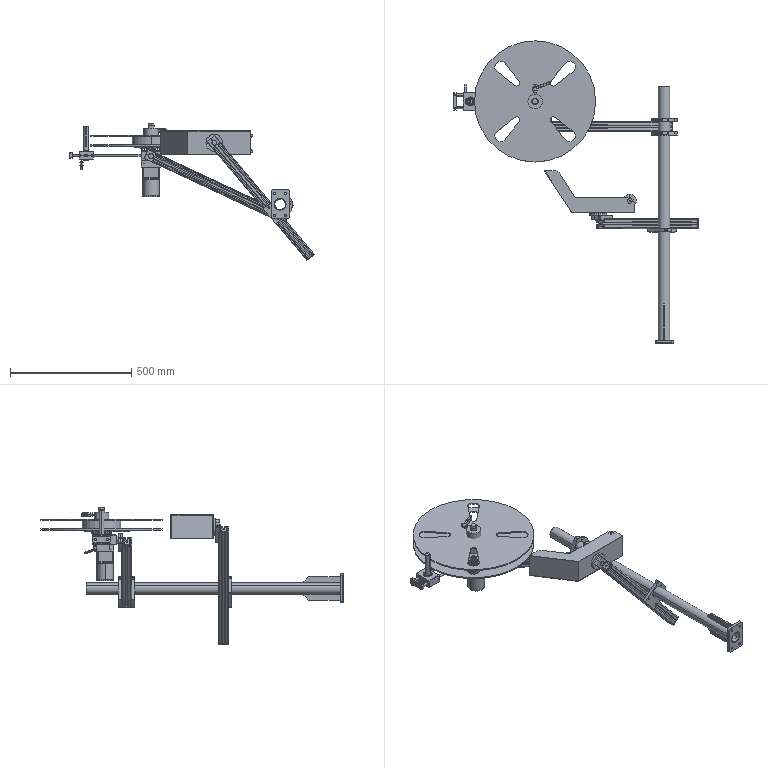Part | NX | 43 solids | 1494 faces | box 1008 x 1246 x 564.853 mm | volume 6126182 mm3 | cylinder 582 | plane 522 | cone 293 | torus 57 | spline 30 | sphere 10 | commonest cylinder face diameters 4.2 x44 10 x39 8 x36 6.5 x28 25 x28 19 x26